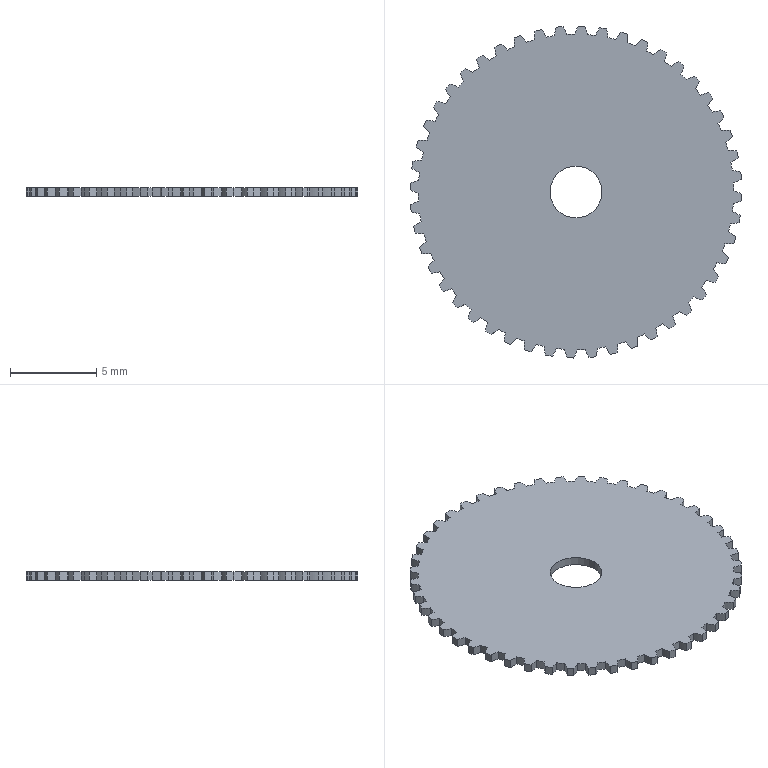Part | SolidWorks | features CirPattern 1, Cut 1, Extrusion 1, ICE 1 | 1 solid | 198 faces | box 19.259 x 19.259 x 0.5 mm | volume 134.631 mm3 | cylinder 196 | plane 2 | commonest cylinder face diameters 6.396 x98 18.3 x48 19.26 x48 3 x2